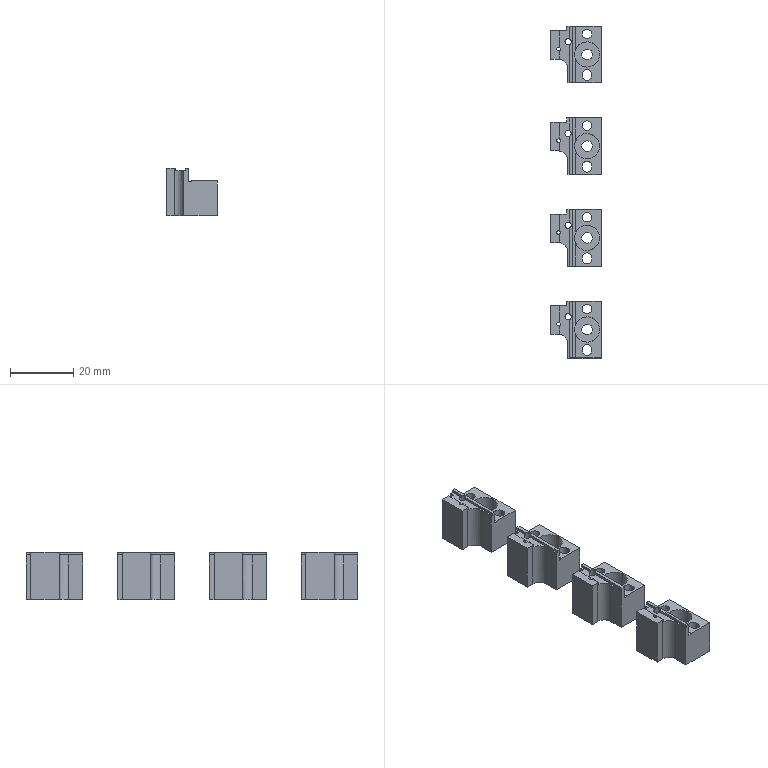Part | 4 solids | 152 faces | box 16 x 105 x 15 mm | volume 8842 mm3 | plane 100 | cylinder 44 | cone 8 | commonest cylinder face diameters 3 x12 2.5 x8 1.2 x4 2 x4 3.05 x4 3.4 x4